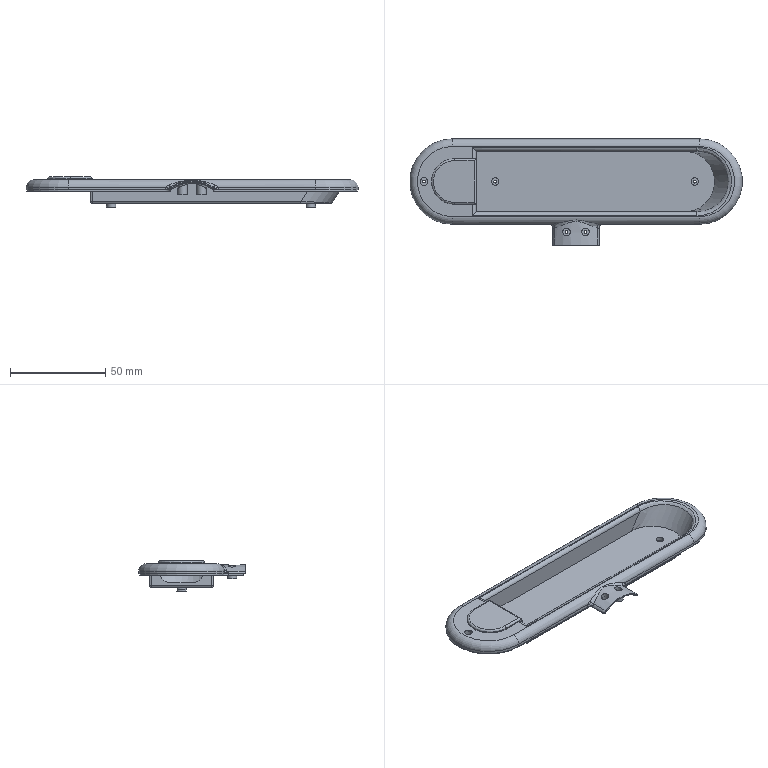Part | NX | features SKETCH 14, BLEND 8, EXTRUDE 8, CBORE_HOLE 5, DATUM_PLANE 3, HOLE PACKAGE 3, DATUM_CSYS 2, SCALE 2, SHELL 2, TRIM BODY 2, UNITE 2, CHAMFER 1, CPROJ 1, EXTRACT_FACE 1, SWP104 1, THRU_CURVE 1, TRIM_AND_EXTEND 1 | 1 solid | 126 faces | box 175 x 56 x 16 mm | volume 12208 mm3 | cylinder 51 | plane 44 | spline 17 | torus 9 | cone 3 | sphere 2 | commonest cylinder face diameters 2 x10 4 x9 5 x9 1.5 x5 3 x2 6 x2